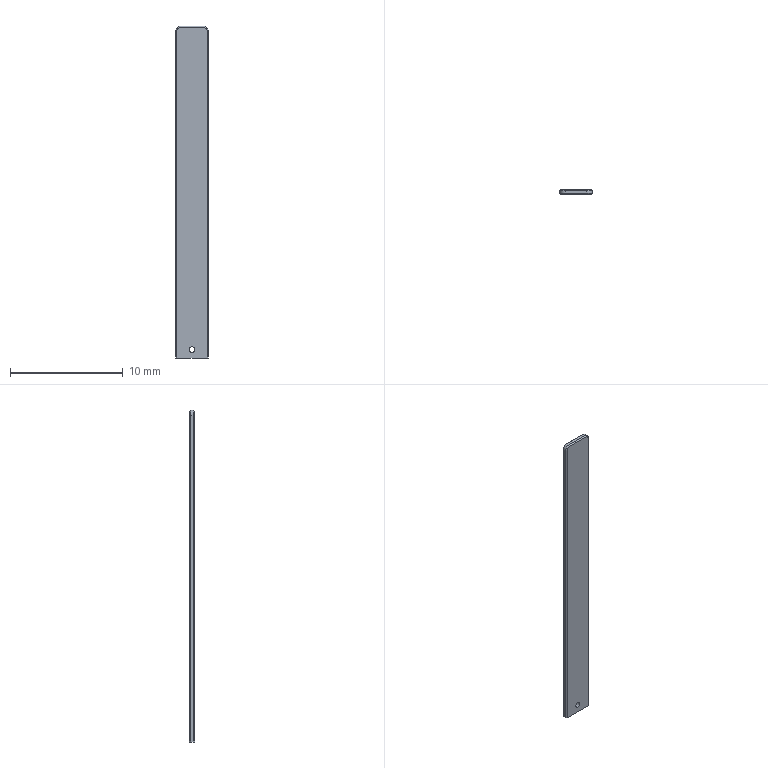Part | SolidWorks | features ICE 6, Chamfer 2, Extrusion 1, Fillet 1 | 1 solid | 20 faces | box 2.9 x 0.45 x 29.5 mm | volume 37.747 mm3 | plane 12 | cylinder 4 | cone 4 | commonest cylinder face diameters 0.5 x2 1 x2
STEP:
#1=CARTESIAN_POINT('',(0.,0.65,-0.5));
#2=VERTEX_POINT('',#1);
#3=CARTESIAN_POINT('',(0.,0.65,-1.));
#4=VERTEX_POINT('',#3);
#5=CARTESIAN_POINT('',(0.,0.65,-0.75));
#6=DIRECTION('',(0.,-1.,0.));
#7=DIRECTION('',(1.,0.,0.));
#8=AXIS2_PLACEMENT_3D('',#5,#6,#7);
#9=CIRCLE('',#8,0.25);
#10=EDGE_CURVE('',#2,#4,#9,.T.);
#11=ORIENTED_EDGE('',*,*,#10,.F.);
#12=CARTESIAN_POINT('',(0.,0.2,-0.5));
#13=VERTEX_POINT('',#12);
#14=CARTESIAN_POINT('',(0.,3.2,-0.5));
#15=DIRECTION('',(0.,-1.,0.));
#16=VECTOR('',#15,1000.);
#17=LINE('',#14,#16);
#18=EDGE_CURVE('',#2,#13,#17,.T.);
#19=ORIENTED_EDGE('',*,*,#18,.T.);
#20=CARTESIAN_POINT('',(0.,0.2,-1.));
#21=VERTEX_POINT('',#20);
#22=CARTESIAN_POINT('',(0.,0.2,-0.75));
#23=DIRECTION('',(0.,-1.,0.));
#24=DIRECTION('',(0.,0.,-1.));
#25=AXIS2_PLACEMENT_3D('',#22,#23,#24);
#26=CIRCLE('',#25,0.25);
#27=EDGE_CURVE('',#13,#21,#26,.T.);
#28=ORIENTED_EDGE('',*,*,#27,.T.);
#29=CARTESIAN_POINT('',(0.,3.2,-1.));
#30=DIRECTION('',(0.,-1.,0.));
#31=VECTOR('',#30,1000.);
#32=LINE('',#29,#31);
#33=EDGE_CURVE('',#4,#21,#32,.T.);
#34=ORIENTED_EDGE('',*,*,#33,.F.);
#35=EDGE_LOOP('',(#11,#19,#28,#34));
#36=FACE_OUTER_BOUND('',#35,.T.);
#37=CARTESIAN_POINT('',(0.,3.2,-0.75));
#38=DIRECTION('',(0.,-1.,0.));
#39=DIRECTION('',(0.,0.,-1.));
#40=AXIS2_PLACEMENT_3D('',#37,#38,#39);
#41=CYLINDRICAL_SURFACE('',#40,0.25);
#42=ADVANCED_FACE('',(#36),#41,.F.);
#43=CARTESIAN_POINT('',(1.45,0.3,27.5));
#44=VERTEX_POINT('',#43);
#45=CARTESIAN_POINT('',(1.45,0.3,-1.5));
#46=VERTEX_POINT('',#45);
#47=CARTESIAN_POINT('',(1.45,0.3,28.));
#48=DIRECTION('',(0.,0.,-1.));
#49=VECTOR('',#48,1000.);
#50=LINE('',#47,#49);
#51=EDGE_CURVE('',#44,#46,#50,.T.);
#52=ORIENTED_EDGE('',*,*,#51,.T.);
#53=CARTESIAN_POINT('',(1.45,0.55,-1.5));
#54=VERTEX_POINT('',#53);
#55=CARTESIAN_POINT('',(1.45,0.55,-1.5));
#56=DIRECTION('',(0.,-1.,0.));
#57=VECTOR('',#56,1000.);
#58=LINE('',#55,#57);
#59=EDGE_CURVE('',#54,#46,#58,.T.);
#60=ORIENTED_EDGE('',*,*,#59,.F.);
#61=CARTESIAN_POINT('',(1.45,0.55,27.5));
#62=VERTEX_POINT('',#61);
#63=CARTESIAN_POINT('',(1.45,0.55,28.));
#64=DIRECTION('',(0.,0.,1.));
#65=VECTOR('',#64,1000.);
#66=LINE('',#63,#65);
#67=EDGE_CURVE('',#54,#62,#66,.T.);
#68=ORIENTED_EDGE('',*,*,#67,.T.);
#69=CARTESIAN_POINT('',(1.45,0.2,27.5));
#70=DIRECTION('',(0.,-1.,0.));
#71=VECTOR('',#70,1000.);
#72=LINE('',#69,#71);
#73=EDGE_CURVE('',#62,#44,#72,.T.);
#74=ORIENTED_EDGE('',*,*,#73,.T.);
#75=EDGE_LOOP('',(#52,#60,#68,#74));
#76=FACE_OUTER_BOUND('',#75,.T.);
#77=CARTESIAN_POINT('',(1.45,0.65,28.));
#78=DIRECTION('',(-1.,0.,0.));
#79=DIRECTION('',(0.,0.,1.));
#80=AXIS2_PLACEMENT_3D('',#77,#78,#79);
#81=PLANE('',#80);
#82=ADVANCED_FACE('',(#76),#81,.F.);
#83=CARTESIAN_POINT('',(0.,0.65,-0.75));
#84=DIRECTION('',(0.,-1.,0.));
#85=DIRECTION('',(1.,0.,0.));
#86=AXIS2_PLACEMENT_3D('',#83,#84,#85);
#87=CIRCLE('',#86,0.25);
#88=EDGE_CURVE('',#4,#2,#87,.T.);
#89=ORIENTED_EDGE('',*,*,#88,.T.);
#90=ORIENTED_EDGE('',*,*,#10,.T.);
#91=EDGE_LOOP('',(#89,#90));
#92=FACE_BOUND('',#91,.T.);
#93=CARTESIAN_POINT('',(0.95,0.65,27.9));
#94=VERTEX_POINT('',#93);
#95=CARTESIAN_POINT('',(1.35,0.65,27.5));
#96=VERTEX_POINT('',#95);
#97=CARTESIAN_POINT('',(0.95,0.65,27.5));
#98=DIRECTION('',(0.,1.,0.));
#99=DIRECTION('',(1.,0.,0.));
#100=AXIS2_PLACEMENT_3D('',#97,#98,#99);
#101=CIRCLE('',#100,0.4);
#102=EDGE_CURVE('',#94,#96,#101,.T.);
#103=ORIENTED_EDGE('',*,*,#102,.T.);
#104=CARTESIAN_POINT('',(1.35,0.65,-1.5));
#105=VERTEX_POINT('',#104);
#106=CARTESIAN_POINT('',(1.35,0.65,28.));
#107=DIRECTION('',(0.,0.,-1.));
#108=VECTOR('',#107,1000.);
#109=LINE('',#106,#108);
#110=EDGE_CURVE('',#96,#105,#109,.T.);
#111=ORIENTED_EDGE('',*,*,#110,.T.);
#112=CARTESIAN_POINT('',(-1.35,0.65,-1.5));
#113=VERTEX_POINT('',#112);
#114=CARTESIAN_POINT('',(-1.35,0.65,-1.5));
#115=DIRECTION('',(1.,0.,0.));
#116=VECTOR('',#115,1000.);
#117=LINE('',#114,#116);
#118=EDGE_CURVE('',#113,#105,#117,.T.);
#119=ORIENTED_EDGE('',*,*,#118,.F.);
#120=CARTESIAN_POINT('',(-1.35,0.65,27.5));
#121=VERTEX_POINT('',#120);
#122=CARTESIAN_POINT('',(-1.35,0.65,28.));
#123=DIRECTION('',(0.,0.,1.));
#124=VECTOR('',#123,1000.);
#125=LINE('',#122,#124);
#126=EDGE_CURVE('',#113,#121,#125,.T.);
#127=ORIENTED_EDGE('',*,*,#126,.T.);
#128=CARTESIAN_POINT('',(-0.95,0.65,27.9));
#129=VERTEX_POINT('',#128);
#130=CARTESIAN_POINT('',(-0.95,0.65,27.5));
#131=DIRECTION('',(0.,1.,0.));
#132=DIRECTION('',(1.,0.,0.));
#133=AXIS2_PLACEMENT_3D('',#130,#131,#132);
#134=CIRCLE('',#133,0.4);
#135=EDGE_CURVE('',#121,#129,#134,.T.);
#136=ORIENTED_EDGE('',*,*,#135,.T.);
#137=CARTESIAN_POINT('',(0.95,0.65,27.9));
#138=DIRECTION('',(1.,0.,0.));
#139=VECTOR('',#138,1000.);
#140=LINE('',#137,#139);
#141=EDGE_CURVE('',#129,#94,#140,.T.);
#142=ORIENTED_EDGE('',*,*,#141,.T.);
#143=EDGE_LOOP('',(#103,#111,#119,#127,#136,#142));
#144=FACE_OUTER_BOUND('',#143,.T.);
#145=CARTESIAN_POINT('',(-1.45,0.65,28.));
#146=DIRECTION('',(0.,-1.,0.));
#147=DIRECTION('',(1.,0.,0.));
#148=AXIS2_PLACEMENT_3D('',#145,#146,#147);
#149=PLANE('',#148);
#150=ADVANCED_FACE('',(#92,#144),#149,.F.);
#151=CARTESIAN_POINT('',(-1.45,0.3,27.5));
#152=VERTEX_POINT('',#151);
#153=CARTESIAN_POINT('',(-1.45,0.55,27.5));
#154=VERTEX_POINT('',#153);
#155=CARTESIAN_POINT('',(-1.45,0.65,27.5));
#156=DIRECTION('',(0.,1.,0.));
#157=VECTOR('',#156,1000.);
#158=LINE('',#155,#157);
#159=EDGE_CURVE('',#152,#154,#158,.T.);
#160=ORIENTED_EDGE('',*,*,#159,.T.);
#161=CARTESIAN_POINT('',(-1.45,0.55,-1.5));
#162=VERTEX_POINT('',#161);
#163=CARTESIAN_POINT('',(-1.45,0.55,28.));
#164=DIRECTION('',(0.,0.,-1.));
#165=VECTOR('',#164,1000.);
#166=LINE('',#163,#165);
#167=EDGE_CURVE('',#154,#162,#166,.T.);
#168=ORIENTED_EDGE('',*,*,#167,.T.);
#169=CARTESIAN_POINT('',(-1.45,0.3,-1.5));
#170=VERTEX_POINT('',#169);
#171=CARTESIAN_POINT('',(-1.45,0.3,-1.5));
#172=DIRECTION('',(0.,1.,0.));
#173=VECTOR('',#172,1000.);
#174=LINE('',#171,#173);
#175=EDGE_CURVE('',#170,#162,#174,.T.);
#176=ORIENTED_EDGE('',*,*,#175,.F.);
#177=CARTESIAN_POINT('',(-1.45,0.3,28.));
#178=DIRECTION('',(0.,0.,1.));
#179=VECTOR('',#178,1000.);
#180=LINE('',#177,#179);
#181=EDGE_CURVE('',#170,#152,#180,.T.);
#182=ORIENTED_EDGE('',*,*,#181,.T.);
#183=EDGE_LOOP('',(#160,#168,#176,#182));
#184=FACE_OUTER_BOUND('',#183,.T.);
#185=CARTESIAN_POINT('',(-1.45,0.65,28.));
#186=DIRECTION('',(1.,0.,0.));
#187=DIRECTION('',(0.,1.,0.));
#188=AXIS2_PLACEMENT_3D('',#185,#186,#187);
#189=PLANE('',#188);
#190=ADVANCED_FACE('',(#184),#189,.F.);
#191=CARTESIAN_POINT('',(0.,0.2,-0.75));
#192=DIRECTION('',(0.,-1.,0.));
#193=DIRECTION('',(0.,0.,-1.));
#194=AXIS2_PLACEMENT_3D('',#191,#192,#193);
#195=CIRCLE('',#194,0.25);
#196=EDGE_CURVE('',#21,#13,#195,.T.);
#197=ORIENTED_EDGE('',*,*,#196,.F.);
#198=ORIENTED_EDGE('',*,*,#27,.F.);
#199=EDGE_LOOP('',(#197,#198));
#200=FACE_BOUND('',#199,.T.);
#201=CARTESIAN_POINT('',(-1.35,0.2,27.5));
#202=VERTEX_POINT('',#201);
#203=CARTESIAN_POINT('',(-1.35,0.2,-1.5));
#204=VERTEX_POINT('',#203);
#205=CARTESIAN_POINT('',(-1.35,0.2,28.));
#206=DIRECTION('',(0.,0.,-1.));
#207=VECTOR('',#206,1000.);
#208=LINE('',#205,#207);
#209=EDGE_CURVE('',#202,#204,#208,.T.);
#210=ORIENTED_EDGE('',*,*,#209,.T.);
#211=CARTESIAN_POINT('',(1.35,0.2,-1.5));
#212=VERTEX_POINT('',#211);
#213=CARTESIAN_POINT('',(1.35,0.2,-1.5));
#214=DIRECTION('',(-1.,0.,0.));
#215=VECTOR('',#214,1000.);
#216=LINE('',#213,#215);
#217=EDGE_CURVE('',#212,#204,#216,.T.);
#218=ORIENTED_EDGE('',*,*,#217,.F.);
#219=CARTESIAN_POINT('',(1.35,0.2,27.5));
#220=VERTEX_POINT('',#219);
#221=CARTESIAN_POINT('',(1.35,0.2,28.));
#222=DIRECTION('',(0.,0.,1.));
#223=VECTOR('',#222,1000.);
#224=LINE('',#221,#223);
#225=EDGE_CURVE('',#212,#220,#224,.T.);
#226=ORIENTED_EDGE('',*,*,#225,.T.);
#227=CARTESIAN_POINT('',(0.95,0.2,27.9));
#228=VERTEX_POINT('',#227);
#229=CARTESIAN_POINT('',(0.95,0.2,27.5));
#230=DIRECTION('',(0.,-1.,0.));
#231=DIRECTION('',(0.,0.,1.));
#232=AXIS2_PLACEMENT_3D('',#229,#230,#231);
#233=CIRCLE('',#232,0.4);
#234=EDGE_CURVE('',#220,#228,#233,.T.);
#235=ORIENTED_EDGE('',*,*,#234,.T.);
#236=CARTESIAN_POINT('',(-0.95,0.2,27.9));
#237=VERTEX_POINT('',#236);
#238=CARTESIAN_POINT('',(-0.95,0.2,27.9));
#239=DIRECTION('',(-1.,0.,0.));
#240=VECTOR('',#239,1000.);
#241=LINE('',#238,#240);
#242=EDGE_CURVE('',#228,#237,#241,.T.);
#243=ORIENTED_EDGE('',*,*,#242,.T.);
#244=CARTESIAN_POINT('',(-0.95,0.2,27.5));
#245=DIRECTION('',(0.,-1.,0.));
#246=DIRECTION('',(0.,0.,1.));
#247=AXIS2_PLACEMENT_3D('',#244,#245,#246);
#248=CIRCLE('',#247,0.4);
#249=EDGE_CURVE('',#237,#202,#248,.T.);
#250=ORIENTED_EDGE('',*,*,#249,.T.);
#251=EDGE_LOOP('',(#210,#218,#226,#235,#243,#250));
#252=FACE_OUTER_BOUND('',#251,.T.);
#253=CARTESIAN_POINT('',(-1.45,0.2,28.));
#254=DIRECTION('',(0.,1.,0.));
#255=DIRECTION('',(0.,0.,1.));
#256=AXIS2_PLACEMENT_3D('',#253,#254,#255);
#257=PLANE('',#256);
#258=ADVANCED_FACE('',(#200,#252),#257,.F.);
#259=CARTESIAN_POINT('',(0.95,0.3,28.));
#260=VERTEX_POINT('',#259);
#261=CARTESIAN_POINT('',(0.95,0.55,28.));
#262=VERTEX_POINT('',#261);
#263=CARTESIAN_POINT('',(0.95,0.65,28.));
#264=DIRECTION('',(0.,1.,0.));
#265=VECTOR('',#264,1000.);
#266=LINE('',#263,#265);
#267=EDGE_CURVE('',#260,#262,#266,.T.);
#268=ORIENTED_EDGE('',*,*,#267,.T.);
#269=CARTESIAN_POINT('',(-0.95,0.55,28.));
#270=VERTEX_POINT('',#269);
#271=CARTESIAN_POINT('',(-0.95,0.55,28.));
#272=DIRECTION('',(-1.,0.,0.));
#273=VECTOR('',#272,1000.);
#274=LINE('',#271,#273);
#275=EDGE_CURVE('',#262,#270,#274,.T.);
#276=ORIENTED_EDGE('',*,*,#275,.T.);
#277=CARTESIAN_POINT('',(-0.95,0.3,28.));
#278=VERTEX_POINT('',#277);
#279=CARTESIAN_POINT('',(-0.95,0.2,28.));
#280=DIRECTION('',(0.,-1.,0.));
#281=VECTOR('',#280,1000.);
#282=LINE('',#279,#281);
#283=EDGE_CURVE('',#270,#278,#282,.T.);
#284=ORIENTED_EDGE('',*,*,#283,.T.);
#285=CARTESIAN_POINT('',(0.95,0.3,28.));
#286=DIRECTION('',(1.,0.,0.));
#287=VECTOR('',#286,1000.);
#288=LINE('',#285,#287);
#289=EDGE_CURVE('',#278,#260,#288,.T.);
#290=ORIENTED_EDGE('',*,*,#289,.T.);
#291=EDGE_LOOP('',(#268,#276,#284,#290));
#292=FACE_OUTER_BOUND('',#291,.T.);
#293=CARTESIAN_POINT('',(0.,0.,28.));
#294=DIRECTION('',(0.,0.,1.));
#295=DIRECTION('',(1.,0.,0.));
#296=AXIS2_PLACEMENT_3D('',#293,#294,#295);
#297=PLANE('',#296);
#298=ADVANCED_FACE('',(#292),#297,.T.);
#299=ORIENTED_EDGE('',*,*,#283,.F.);
#300=CARTESIAN_POINT('',(-0.95,0.55,27.5));
#301=DIRECTION('',(0.,-1.,0.));
#302=DIRECTION('',(1.,0.,0.));
#303=AXIS2_PLACEMENT_3D('',#300,#301,#302);
#304=CIRCLE('',#303,0.5);
#305=EDGE_CURVE('',#270,#154,#304,.T.);
#306=ORIENTED_EDGE('',*,*,#305,.T.);
#307=ORIENTED_EDGE('',*,*,#159,.F.);
#308=CARTESIAN_POINT('',(-0.95,0.3,27.5));
#309=DIRECTION('',(0.,1.,0.));
#310=DIRECTION('',(0.,0.,1.));
#311=AXIS2_PLACEMENT_3D('',#308,#309,#310);
#312=CIRCLE('',#311,0.5);
#313=EDGE_CURVE('',#152,#278,#312,.T.);
#314=ORIENTED_EDGE('',*,*,#313,.T.);
#315=EDGE_LOOP('',(#299,#306,#307,#314));
#316=FACE_OUTER_BOUND('',#315,.T.);
#317=CARTESIAN_POINT('',(-0.95,0.,27.5));
#318=DIRECTION('',(0.,1.,0.));
#319=DIRECTION('',(-1.,0.,0.));
#320=AXIS2_PLACEMENT_3D('',#317,#318,#319);
#321=CYLINDRICAL_SURFACE('',#320,0.5);
#322=ADVANCED_FACE('',(#316),#321,.T.);
#323=ORIENTED_EDGE('',*,*,#73,.F.);
#324=CARTESIAN_POINT('',(0.95,0.55,27.5));
#325=DIRECTION('',(0.,-1.,0.));
#326=DIRECTION('',(0.,0.,-1.));
#327=AXIS2_PLACEMENT_3D('',#324,#325,#326);
#328=CIRCLE('',#327,0.5);
#329=EDGE_CURVE('',#62,#262,#328,.T.);
#330=ORIENTED_EDGE('',*,*,#329,.T.);
#331=ORIENTED_EDGE('',*,*,#267,.F.);
#332=CARTESIAN_POINT('',(0.95,0.3,27.5));
#333=DIRECTION('',(0.,1.,0.));
#334=DIRECTION('',(0.,0.,1.));
#335=AXIS2_PLACEMENT_3D('',#332,#333,#334);
#336=CIRCLE('',#335,0.5);
#337=EDGE_CURVE('',#260,#44,#336,.T.);
#338=ORIENTED_EDGE('',*,*,#337,.T.);
#339=EDGE_LOOP('',(#323,#330,#331,#338));
#340=FACE_OUTER_BOUND('',#339,.T.);
#341=CARTESIAN_POINT('',(0.95,0.,27.5));
#342=DIRECTION('',(0.,-1.,0.));
#343=DIRECTION('',(0.,0.,-1.));
#344=AXIS2_PLACEMENT_3D('',#341,#342,#343);
#345=CYLINDRICAL_SURFACE('',#344,0.5);
#346=ADVANCED_FACE('',(#340),#345,.T.);
#347=ORIENTED_EDGE('',*,*,#126,.F.);
#348=CARTESIAN_POINT('',(-1.45,0.55,-1.5));
#349=DIRECTION('',(0.7071,0.7071,0.));
#350=VECTOR('',#349,1000.);
#351=LINE('',#348,#350);
#352=EDGE_CURVE('',#162,#113,#351,.T.);
#353=ORIENTED_EDGE('',*,*,#352,.F.);
#354=ORIENTED_EDGE('',*,*,#167,.F.);
#355=CARTESIAN_POINT('',(-1.35,0.65,27.5));
#356=DIRECTION('',(-0.7071,-0.7071,0.));
#357=VECTOR('',#356,1000.);
#358=LINE('',#355,#357);
#359=EDGE_CURVE('',#121,#154,#358,.T.);
#360=ORIENTED_EDGE('',*,*,#359,.F.);
#361=EDGE_LOOP('',(#347,#353,#354,#360));
#362=FACE_OUTER_BOUND('',#361,.T.);
#363=CARTESIAN_POINT('',(-1.45,0.55,28.));
#364=DIRECTION('',(0.7071,-0.7071,0.));
#365=DIRECTION('',(0.,0.,-1.));
#366=AXIS2_PLACEMENT_3D('',#363,#364,#365);
#367=PLANE('',#366);
#368=ADVANCED_FACE('',(#362),#367,.F.);
#369=ORIENTED_EDGE('',*,*,#359,.T.);
#370=ORIENTED_EDGE('',*,*,#305,.F.);
#371=CARTESIAN_POINT('',(-0.95,0.65,27.9));
#372=DIRECTION('',(0.,-0.7071,0.7071));
#373=VECTOR('',#372,1000.);
#374=LINE('',#371,#373);
#375=EDGE_CURVE('',#129,#270,#374,.T.);
#376=ORIENTED_EDGE('',*,*,#375,.F.);
#377=ORIENTED_EDGE('',*,*,#135,.F.);
#378=EDGE_LOOP('',(#369,#370,#376,#377));
#379=FACE_OUTER_BOUND('',#378,.T.);
#380=CARTESIAN_POINT('',(-0.95,0.65,27.5));
#381=DIRECTION('',(0.,-1.,0.));
#382=DIRECTION('',(1.,0.,0.));
#383=AXIS2_PLACEMENT_3D('',#380,#381,#382);
#384=CONICAL_SURFACE('',#383,0.4,0.7854);
#385=ADVANCED_FACE('',(#379),#384,.T.);
#386=ORIENTED_EDGE('',*,*,#375,.T.);
#387=ORIENTED_EDGE('',*,*,#275,.F.);
#388=CARTESIAN_POINT('',(0.95,0.65,27.9));
#389=DIRECTION('',(0.,-0.7071,0.7071));
#390=VECTOR('',#389,1000.);
#391=LINE('',#388,#390);
#392=EDGE_CURVE('',#94,#262,#391,.T.);
#393=ORIENTED_EDGE('',*,*,#392,.F.);
#394=ORIENTED_EDGE('',*,*,#141,.F.);
#395=EDGE_LOOP('',(#386,#387,#393,#394));
#396=FACE_OUTER_BOUND('',#395,.T.);
#397=CARTESIAN_POINT('',(0.,0.55,28.));
#398=DIRECTION('',(0.,0.7071,0.7071));
#399=DIRECTION('',(1.,0.,0.));
#400=AXIS2_PLACEMENT_3D('',#397,#398,#399);
#401=PLANE('',#400);
#402=ADVANCED_FACE('',(#396),#401,.T.);
#403=ORIENTED_EDGE('',*,*,#392,.T.);
#404=ORIENTED_EDGE('',*,*,#329,.F.);
#405=CARTESIAN_POINT('',(1.35,0.65,27.5));
#406=DIRECTION('',(0.7071,-0.7071,0.));
#407=VECTOR('',#406,1000.);
#408=LINE('',#405,#407);
#409=EDGE_CURVE('',#96,#62,#408,.T.);
#410=ORIENTED_EDGE('',*,*,#409,.F.);
#411=ORIENTED_EDGE('',*,*,#102,.F.);
#412=EDGE_LOOP('',(#403,#404,#410,#411));
#413=FACE_OUTER_BOUND('',#412,.T.);
#414=CARTESIAN_POINT('',(0.95,0.65,27.5));
#415=DIRECTION('',(0.,-1.,0.));
#416=DIRECTION('',(0.,0.,-1.));
#417=AXIS2_PLACEMENT_3D('',#414,#415,#416);
#418=CONICAL_SURFACE('',#417,0.4,0.7854);
#419=ADVANCED_FACE('',(#413),#418,.T.);
#420=ORIENTED_EDGE('',*,*,#409,.T.);
#421=ORIENTED_EDGE('',*,*,#67,.F.);
#422=CARTESIAN_POINT('',(1.35,0.65,-1.5));
#423=DIRECTION('',(0.7071,-0.7071,0.));
#424=VECTOR('',#423,1000.);
#425=LINE('',#422,#424);
#426=EDGE_CURVE('',#105,#54,#425,.T.);
#427=ORIENTED_EDGE('',*,*,#426,.F.);
#428=ORIENTED_EDGE('',*,*,#110,.F.);
#429=EDGE_LOOP('',(#420,#421,#427,#428));
#430=FACE_OUTER_BOUND('',#429,.T.);
#431=CARTESIAN_POINT('',(1.35,0.65,28.));
#432=DIRECTION('',(-0.7071,-0.7071,0.));
#433=DIRECTION('',(0.,0.,-1.));
#434=AXIS2_PLACEMENT_3D('',#431,#432,#433);
#435=PLANE('',#434);
#436=ADVANCED_FACE('',(#430),#435,.F.);
#437=ORIENTED_EDGE('',*,*,#181,.F.);
#438=CARTESIAN_POINT('',(-1.35,0.2,-1.5));
#439=DIRECTION('',(-0.7071,0.7071,0.));
#440=VECTOR('',#439,1000.);
#441=LINE('',#438,#440);
#442=EDGE_CURVE('',#204,#170,#441,.T.);
#443=ORIENTED_EDGE('',*,*,#442,.F.);
#444=ORIENTED_EDGE('',*,*,#209,.F.);
#445=CARTESIAN_POINT('',(-1.45,0.3,27.5));
#446=DIRECTION('',(0.7071,-0.7071,0.));
#447=VECTOR('',#446,1000.);
#448=LINE('',#445,#447);
#449=EDGE_CURVE('',#152,#202,#448,.T.);
#450=ORIENTED_EDGE('',*,*,#449,.F.);
#451=EDGE_LOOP('',(#437,#443,#444,#450));
#452=FACE_OUTER_BOUND('',#451,.T.);
#453=CARTESIAN_POINT('',(-1.35,0.2,28.));
#454=DIRECTION('',(0.7071,0.7071,0.));
#455=DIRECTION('',(0.,0.,-1.));
#456=AXIS2_PLACEMENT_3D('',#453,#454,#455);
#457=PLANE('',#456);
#458=ADVANCED_FACE('',(#452),#457,.F.);
#459=ORIENTED_EDGE('',*,*,#449,.T.);
#460=ORIENTED_EDGE('',*,*,#249,.F.);
#461=CARTESIAN_POINT('',(-0.95,0.3,28.));
#462=DIRECTION('',(0.,-0.7071,-0.7071));
#463=VECTOR('',#462,1000.);
#464=LINE('',#461,#463);
#465=EDGE_CURVE('',#278,#237,#464,.T.);
#466=ORIENTED_EDGE('',*,*,#465,.F.);
#467=ORIENTED_EDGE('',*,*,#313,.F.);
#468=EDGE_LOOP('',(#459,#460,#466,#467));
#469=FACE_OUTER_BOUND('',#468,.T.);
#470=CARTESIAN_POINT('',(-0.95,0.2,27.5));
#471=DIRECTION('',(0.,1.,0.));
#472=DIRECTION('',(0.,0.,1.));
#473=AXIS2_PLACEMENT_3D('',#470,#471,#472);
#474=CONICAL_SURFACE('',#473,0.4,0.7854);
#475=ADVANCED_FACE('',(#469),#474,.T.);
#476=ORIENTED_EDGE('',*,*,#465,.T.);
#477=ORIENTED_EDGE('',*,*,#242,.F.);
#478=CARTESIAN_POINT('',(0.95,0.3,28.));
#479=DIRECTION('',(0.,-0.7071,-0.7071));
#480=VECTOR('',#479,1000.);
#481=LINE('',#478,#480);
#482=EDGE_CURVE('',#260,#228,#481,.T.);
#483=ORIENTED_EDGE('',*,*,#482,.F.);
#484=ORIENTED_EDGE('',*,*,#289,.F.);
#485=EDGE_LOOP('',(#476,#477,#483,#484));
#486=FACE_OUTER_BOUND('',#485,.T.);
#487=CARTESIAN_POINT('',(0.,0.3,28.));
#488=DIRECTION('',(0.,-0.7071,0.7071));
#489=DIRECTION('',(-1.,0.,0.));
#490=AXIS2_PLACEMENT_3D('',#487,#488,#489);
#491=PLANE('',#490);
#492=ADVANCED_FACE('',(#486),#491,.T.);
#493=ORIENTED_EDGE('',*,*,#482,.T.);
#494=ORIENTED_EDGE('',*,*,#234,.F.);
#495=CARTESIAN_POINT('',(1.45,0.3,27.5));
#496=DIRECTION('',(-0.7071,-0.7071,0.));
#497=VECTOR('',#496,1000.);
#498=LINE('',#495,#497);
#499=EDGE_CURVE('',#44,#220,#498,.T.);
#500=ORIENTED_EDGE('',*,*,#499,.F.);
#501=ORIENTED_EDGE('',*,*,#337,.F.);
#502=EDGE_LOOP('',(#493,#494,#500,#501));
#503=FACE_OUTER_BOUND('',#502,.T.);
#504=CARTESIAN_POINT('',(0.95,0.2,27.5));
#505=DIRECTION('',(0.,1.,0.));
#506=DIRECTION('',(0.,0.,1.));
#507=AXIS2_PLACEMENT_3D('',#504,#505,#506);
#508=CONICAL_SURFACE('',#507,0.4,0.7854);
#509=ADVANCED_FACE('',(#503),#508,.T.);
#510=ORIENTED_EDGE('',*,*,#499,.T.);
#511=ORIENTED_EDGE('',*,*,#225,.F.);
#512=CARTESIAN_POINT('',(1.45,0.3,-1.5));
#513=DIRECTION('',(-0.7071,-0.7071,0.));
#514=VECTOR('',#513,1000.);
#515=LINE('',#512,#514);
#516=EDGE_CURVE('',#46,#212,#515,.T.);
#517=ORIENTED_EDGE('',*,*,#516,.F.);
#518=ORIENTED_EDGE('',*,*,#51,.F.);
#519=EDGE_LOOP('',(#510,#511,#517,#518));
#520=FACE_OUTER_BOUND('',#519,.T.);
#521=CARTESIAN_POINT('',(1.45,0.3,28.));
#522=DIRECTION('',(-0.7071,0.7071,0.));
#523=DIRECTION('',(0.,0.,-1.));
#524=AXIS2_PLACEMENT_3D('',#521,#522,#523);
#525=PLANE('',#524);
#526=ADVANCED_FACE('',(#520),#525,.F.);
#527=ORIENTED_EDGE('',*,*,#175,.T.);
#528=ORIENTED_EDGE('',*,*,#352,.T.);
#529=ORIENTED_EDGE('',*,*,#118,.T.);
#530=ORIENTED_EDGE('',*,*,#426,.T.);
#531=ORIENTED_EDGE('',*,*,#59,.T.);
#532=ORIENTED_EDGE('',*,*,#516,.T.);
#533=ORIENTED_EDGE('',*,*,#217,.T.);
#534=ORIENTED_EDGE('',*,*,#442,.T.);
#535=EDGE_LOOP('',(#527,#528,#529,#530,#531,#532,#533,#534));
#536=FACE_OUTER_BOUND('',#535,.T.);
#537=CARTESIAN_POINT('',(0.,0.,-1.5));
#538=DIRECTION('',(0.,0.,-1.));
#539=DIRECTION('',(-1.,0.,0.));
#540=AXIS2_PLACEMENT_3D('',#537,#538,#539);
#541=PLANE('',#540);
#542=ADVANCED_FACE('',(#536),#541,.T.);
#543=ORIENTED_EDGE('',*,*,#18,.F.);
#544=ORIENTED_EDGE('',*,*,#88,.F.);
#545=ORIENTED_EDGE('',*,*,#33,.T.);
#546=ORIENTED_EDGE('',*,*,#196,.T.);
#547=EDGE_LOOP('',(#543,#544,#545,#546));
#548=FACE_OUTER_BOUND('',#547,.T.);
#549=CARTESIAN_POINT('',(0.,3.2,-0.75));
#550=DIRECTION('',(0.,-1.,0.));
#551=DIRECTION('',(0.,0.,-1.));
#552=AXIS2_PLACEMENT_3D('',#549,#550,#551);
#553=CYLINDRICAL_SURFACE('',#552,0.25);
#554=ADVANCED_FACE('',(#548),#553,.F.);
#555=CLOSED_SHELL('',(#42,#82,#150,#190,#258,#298,#322,#346,#368,#385,#402,#419,#436,#458,#475,#492,#509,#526,#542,#554));
#556=MANIFOLD_SOLID_BREP('',#555);
#557=CARTESIAN_POINT('',(0.,0.,0.));
#558=DIRECTION('',(0.,0.,1.));
#559=DIRECTION('',(1.,0.,0.));
#560=AXIS2_PLACEMENT_3D('',#557,#558,#559);
#561=(LENGTH_UNIT()NAMED_UNIT(*)SI_UNIT(.MILLI.,.METRE.));
#562=UNCERTAINTY_MEASURE_WITH_UNIT(LENGTH_MEASURE(0.00001),#561,'','');
#563=(NAMED_UNIT(*)PLANE_ANGLE_UNIT()SI_UNIT($,.RADIAN.));
#564=(NAMED_UNIT(*)SI_UNIT($,.STERADIAN.)SOLID_ANGLE_UNIT());
#565=(GEOMETRIC_REPRESENTATION_CONTEXT(3)GLOBAL_UNCERTAINTY_ASSIGNED_CONTEXT((#562))GLOBAL_UNIT_ASSIGNED_CONTEXT((#561,#563,#564))REPRESENTATION_CONTEXT('',''));
#566=ADVANCED_BREP_SHAPE_REPRESENTATION('',(#556,#560),#565);